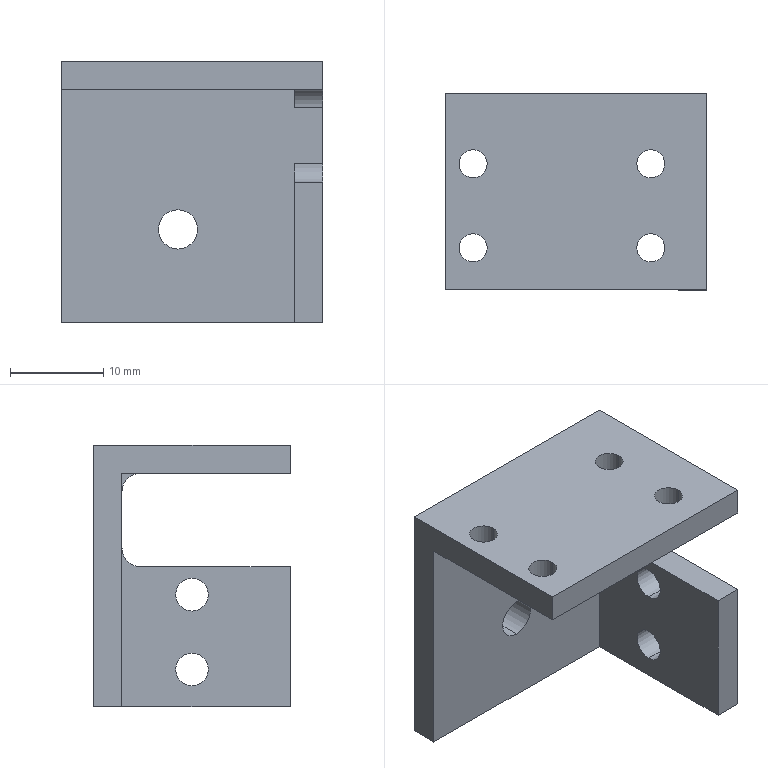Part | SolidWorks | features ICE 2, Extrusion 1 | 1 solid | 28 faces | box 28 x 21 x 28 mm | volume 4495 mm3 | cylinder 16 | plane 12 | commonest cylinder face diameters 3 x8 3.5 x4 4 x2 4.2 x2
STEP:
#1=CARTESIAN_POINT('',(15.5,1.5,-14.75));
#2=VERTEX_POINT('',#1);
#3=CARTESIAN_POINT('',(15.5,1.5,-11.25));
#4=VERTEX_POINT('',#3);
#5=CARTESIAN_POINT('',(15.5,1.5,-13.));
#6=DIRECTION('',(-1.,0.,0.));
#7=DIRECTION('',(0.,0.,1.));
#8=AXIS2_PLACEMENT_3D('',#5,#6,#7);
#9=CIRCLE('',#8,1.75);
#10=EDGE_CURVE('',#2,#4,#9,.T.);
#11=ORIENTED_EDGE('',*,*,#10,.F.);
#12=CARTESIAN_POINT('',(12.5,1.5,-14.75));
#13=VERTEX_POINT('',#12);
#14=CARTESIAN_POINT('',(15.5,1.5,-14.75));
#15=DIRECTION('',(-1.,0.,0.));
#16=VECTOR('',#15,1000.);
#17=LINE('',#14,#16);
#18=EDGE_CURVE('',#2,#13,#17,.T.);
#19=ORIENTED_EDGE('',*,*,#18,.T.);
#20=CARTESIAN_POINT('',(12.5,1.5,-11.25));
#21=VERTEX_POINT('',#20);
#22=CARTESIAN_POINT('',(12.5,1.5,-13.));
#23=DIRECTION('',(-1.,0.,0.));
#24=DIRECTION('',(0.,0.,1.));
#25=AXIS2_PLACEMENT_3D('',#22,#23,#24);
#26=CIRCLE('',#25,1.75);
#27=EDGE_CURVE('',#13,#21,#26,.T.);
#28=ORIENTED_EDGE('',*,*,#27,.T.);
#29=CARTESIAN_POINT('',(15.5,1.5,-11.25));
#30=DIRECTION('',(-1.,0.,0.));
#31=VECTOR('',#30,1000.);
#32=LINE('',#29,#31);
#33=EDGE_CURVE('',#4,#21,#32,.T.);
#34=ORIENTED_EDGE('',*,*,#33,.F.);
#35=EDGE_LOOP('',(#11,#19,#28,#34));
#36=FACE_OUTER_BOUND('',#35,.T.);
#37=CARTESIAN_POINT('',(15.5,1.5,-13.));
#38=DIRECTION('',(-1.,0.,0.));
#39=DIRECTION('',(0.,0.,1.));
#40=AXIS2_PLACEMENT_3D('',#37,#38,#39);
#41=CYLINDRICAL_SURFACE('',#40,1.75);
#42=ADVANCED_FACE('',(#36),#41,.F.);
#43=CARTESIAN_POINT('',(15.5,1.5,-22.75));
#44=VERTEX_POINT('',#43);
#45=CARTESIAN_POINT('',(15.5,1.5,-19.25));
#46=VERTEX_POINT('',#45);
#47=CARTESIAN_POINT('',(15.5,1.5,-21.));
#48=DIRECTION('',(-1.,0.,0.));
#49=DIRECTION('',(0.,0.,1.));
#50=AXIS2_PLACEMENT_3D('',#47,#48,#49);
#51=CIRCLE('',#50,1.75);
#52=EDGE_CURVE('',#44,#46,#51,.T.);
#53=ORIENTED_EDGE('',*,*,#52,.F.);
#54=CARTESIAN_POINT('',(12.5,1.5,-22.75));
#55=VERTEX_POINT('',#54);
#56=CARTESIAN_POINT('',(15.5,1.5,-22.75));
#57=DIRECTION('',(-1.,0.,0.));
#58=VECTOR('',#57,1000.);
#59=LINE('',#56,#58);
#60=EDGE_CURVE('',#44,#55,#59,.T.);
#61=ORIENTED_EDGE('',*,*,#60,.T.);
#62=CARTESIAN_POINT('',(12.5,1.5,-19.25));
#63=VERTEX_POINT('',#62);
#64=CARTESIAN_POINT('',(12.5,1.5,-21.));
#65=DIRECTION('',(-1.,0.,0.));
#66=DIRECTION('',(0.,0.,1.));
#67=AXIS2_PLACEMENT_3D('',#64,#65,#66);
#68=CIRCLE('',#67,1.75);
#69=EDGE_CURVE('',#55,#63,#68,.T.);
#70=ORIENTED_EDGE('',*,*,#69,.T.);
#71=CARTESIAN_POINT('',(15.5,1.5,-19.25));
#72=DIRECTION('',(-1.,0.,0.));
#73=VECTOR('',#72,1000.);
#74=LINE('',#71,#73);
#75=EDGE_CURVE('',#46,#63,#74,.T.);
#76=ORIENTED_EDGE('',*,*,#75,.F.);
#77=EDGE_LOOP('',(#53,#61,#70,#76));
#78=FACE_OUTER_BOUND('',#77,.T.);
#79=CARTESIAN_POINT('',(15.5,1.5,-21.));
#80=DIRECTION('',(-1.,0.,0.));
#81=DIRECTION('',(0.,0.,1.));
#82=AXIS2_PLACEMENT_3D('',#79,#80,#81);
#83=CYLINDRICAL_SURFACE('',#82,1.75);
#84=ADVANCED_FACE('',(#78),#83,.F.);
#85=CARTESIAN_POINT('',(0.,12.,-17.1));
#86=VERTEX_POINT('',#85);
#87=CARTESIAN_POINT('',(0.,12.,-12.9));
#88=VERTEX_POINT('',#87);
#89=CARTESIAN_POINT('',(0.,12.,-15.));
#90=DIRECTION('',(0.,1.,0.));
#91=DIRECTION('',(0.,0.,1.));
#92=AXIS2_PLACEMENT_3D('',#89,#90,#91);
#93=CIRCLE('',#92,2.1);
#94=EDGE_CURVE('',#86,#88,#93,.T.);
#95=ORIENTED_EDGE('',*,*,#94,.T.);
#96=CARTESIAN_POINT('',(0.,9.,-12.9));
#97=VERTEX_POINT('',#96);
#98=CARTESIAN_POINT('',(0.,12.,-12.9));
#99=DIRECTION('',(0.,-1.,0.));
#100=VECTOR('',#99,1000.);
#101=LINE('',#98,#100);
#102=EDGE_CURVE('',#88,#97,#101,.T.);
#103=ORIENTED_EDGE('',*,*,#102,.T.);
#104=CARTESIAN_POINT('',(0.,9.,-17.1));
#105=VERTEX_POINT('',#104);
#106=CARTESIAN_POINT('',(0.,9.,-15.));
#107=DIRECTION('',(0.,1.,0.));
#108=DIRECTION('',(0.,0.,1.));
#109=AXIS2_PLACEMENT_3D('',#106,#107,#108);
#110=CIRCLE('',#109,2.1);
#111=EDGE_CURVE('',#105,#97,#110,.T.);
#112=ORIENTED_EDGE('',*,*,#111,.F.);
#113=CARTESIAN_POINT('',(0.,12.,-17.1));
#114=DIRECTION('',(0.,-1.,0.));
#115=VECTOR('',#114,1000.);
#116=LINE('',#113,#115);
#117=EDGE_CURVE('',#86,#105,#116,.T.);
#118=ORIENTED_EDGE('',*,*,#117,.F.);
#119=EDGE_LOOP('',(#95,#103,#112,#118));
#120=FACE_OUTER_BOUND('',#119,.T.);
#121=CARTESIAN_POINT('',(0.,12.,-15.));
#122=DIRECTION('',(0.,-1.,0.));
#123=DIRECTION('',(0.,0.,-1.));
#124=AXIS2_PLACEMENT_3D('',#121,#122,#123);
#125=CYLINDRICAL_SURFACE('',#124,2.1);
#126=ADVANCED_FACE('',(#120),#125,.F.);
#127=CARTESIAN_POINT('',(-11.,-4.5,3.));
#128=VERTEX_POINT('',#127);
#129=CARTESIAN_POINT('',(-8.,-4.5,3.));
#130=VERTEX_POINT('',#129);
#131=CARTESIAN_POINT('',(-9.5,-4.5,3.));
#132=DIRECTION('',(0.,0.,1.));
#133=DIRECTION('',(1.,0.,0.));
#134=AXIS2_PLACEMENT_3D('',#131,#132,#133);
#135=CIRCLE('',#134,1.5);
#136=EDGE_CURVE('',#128,#130,#135,.T.);
#137=ORIENTED_EDGE('',*,*,#136,.T.);
#138=CARTESIAN_POINT('',(-8.,-4.5,0.));
#139=VERTEX_POINT('',#138);
#140=CARTESIAN_POINT('',(-8.,-4.5,3.));
#141=DIRECTION('',(0.,0.,-1.));
#142=VECTOR('',#141,1000.);
#143=LINE('',#140,#142);
#144=EDGE_CURVE('',#130,#139,#143,.T.);
#145=ORIENTED_EDGE('',*,*,#144,.T.);
#146=CARTESIAN_POINT('',(-11.,-4.5,0.));
#147=VERTEX_POINT('',#146);
#148=CARTESIAN_POINT('',(-9.5,-4.5,0.));
#149=DIRECTION('',(0.,0.,1.));
#150=DIRECTION('',(1.,0.,0.));
#151=AXIS2_PLACEMENT_3D('',#148,#149,#150);
#152=CIRCLE('',#151,1.5);
#153=EDGE_CURVE('',#147,#139,#152,.T.);
#154=ORIENTED_EDGE('',*,*,#153,.F.);
#155=CARTESIAN_POINT('',(-11.,-4.5,3.));
#156=DIRECTION('',(0.,0.,-1.));
#157=VECTOR('',#156,1000.);
#158=LINE('',#155,#157);
#159=EDGE_CURVE('',#128,#147,#158,.T.);
#160=ORIENTED_EDGE('',*,*,#159,.F.);
#161=EDGE_LOOP('',(#137,#145,#154,#160));
#162=FACE_OUTER_BOUND('',#161,.T.);
#163=CARTESIAN_POINT('',(-9.5,-4.5,3.));
#164=DIRECTION('',(0.,0.,-1.));
#165=DIRECTION('',(-1.,0.,0.));
#166=AXIS2_PLACEMENT_3D('',#163,#164,#165);
#167=CYLINDRICAL_SURFACE('',#166,1.5);
#168=ADVANCED_FACE('',(#162),#167,.F.);
#169=CARTESIAN_POINT('',(8.,-4.5,3.));
#170=VERTEX_POINT('',#169);
#171=CARTESIAN_POINT('',(11.,-4.5,3.));
#172=VERTEX_POINT('',#171);
#173=CARTESIAN_POINT('',(9.5,-4.5,3.));
#174=DIRECTION('',(0.,0.,1.));
#175=DIRECTION('',(1.,0.,0.));
#176=AXIS2_PLACEMENT_3D('',#173,#174,#175);
#177=CIRCLE('',#176,1.5);
#178=EDGE_CURVE('',#170,#172,#177,.T.);
#179=ORIENTED_EDGE('',*,*,#178,.T.);
#180=CARTESIAN_POINT('',(11.,-4.5,0.));
#181=VERTEX_POINT('',#180);
#182=CARTESIAN_POINT('',(11.,-4.5,3.));
#183=DIRECTION('',(0.,0.,-1.));
#184=VECTOR('',#183,1000.);
#185=LINE('',#182,#184);
#186=EDGE_CURVE('',#172,#181,#185,.T.);
#187=ORIENTED_EDGE('',*,*,#186,.T.);
#188=CARTESIAN_POINT('',(8.,-4.5,0.));
#189=VERTEX_POINT('',#188);
#190=CARTESIAN_POINT('',(9.5,-4.5,0.));
#191=DIRECTION('',(0.,0.,1.));
#192=DIRECTION('',(1.,0.,0.));
#193=AXIS2_PLACEMENT_3D('',#190,#191,#192);
#194=CIRCLE('',#193,1.5);
#195=EDGE_CURVE('',#189,#181,#194,.T.);
#196=ORIENTED_EDGE('',*,*,#195,.F.);
#197=CARTESIAN_POINT('',(8.,-4.5,3.));
#198=DIRECTION('',(0.,0.,-1.));
#199=VECTOR('',#198,1000.);
#200=LINE('',#197,#199);
#201=EDGE_CURVE('',#170,#189,#200,.T.);
#202=ORIENTED_EDGE('',*,*,#201,.F.);
#203=EDGE_LOOP('',(#179,#187,#196,#202));
#204=FACE_OUTER_BOUND('',#203,.T.);
#205=CARTESIAN_POINT('',(9.5,-4.5,3.));
#206=DIRECTION('',(0.,0.,-1.));
#207=DIRECTION('',(-1.,0.,0.));
#208=AXIS2_PLACEMENT_3D('',#205,#206,#207);
#209=CYLINDRICAL_SURFACE('',#208,1.5);
#210=ADVANCED_FACE('',(#204),#209,.F.);
#211=CARTESIAN_POINT('',(8.,4.5,3.));
#212=VERTEX_POINT('',#211);
#213=CARTESIAN_POINT('',(11.,4.5,3.));
#214=VERTEX_POINT('',#213);
#215=CARTESIAN_POINT('',(9.5,4.5,3.));
#216=DIRECTION('',(0.,0.,1.));
#217=DIRECTION('',(1.,0.,0.));
#218=AXIS2_PLACEMENT_3D('',#215,#216,#217);
#219=CIRCLE('',#218,1.5);
#220=EDGE_CURVE('',#212,#214,#219,.T.);
#221=ORIENTED_EDGE('',*,*,#220,.T.);
#222=CARTESIAN_POINT('',(11.,4.5,0.));
#223=VERTEX_POINT('',#222);
#224=CARTESIAN_POINT('',(11.,4.5,3.));
#225=DIRECTION('',(0.,0.,-1.));
#226=VECTOR('',#225,1000.);
#227=LINE('',#224,#226);
#228=EDGE_CURVE('',#214,#223,#227,.T.);
#229=ORIENTED_EDGE('',*,*,#228,.T.);
#230=CARTESIAN_POINT('',(8.,4.5,0.));
#231=VERTEX_POINT('',#230);
#232=CARTESIAN_POINT('',(9.5,4.5,0.));
#233=DIRECTION('',(0.,0.,1.));
#234=DIRECTION('',(1.,0.,0.));
#235=AXIS2_PLACEMENT_3D('',#232,#233,#234);
#236=CIRCLE('',#235,1.5);
#237=EDGE_CURVE('',#231,#223,#236,.T.);
#238=ORIENTED_EDGE('',*,*,#237,.F.);
#239=CARTESIAN_POINT('',(8.,4.5,3.));
#240=DIRECTION('',(0.,0.,-1.));
#241=VECTOR('',#240,1000.);
#242=LINE('',#239,#241);
#243=EDGE_CURVE('',#212,#231,#242,.T.);
#244=ORIENTED_EDGE('',*,*,#243,.F.);
#245=EDGE_LOOP('',(#221,#229,#238,#244));
#246=FACE_OUTER_BOUND('',#245,.T.);
#247=CARTESIAN_POINT('',(9.5,4.5,3.));
#248=DIRECTION('',(0.,0.,-1.));
#249=DIRECTION('',(-1.,0.,0.));
#250=AXIS2_PLACEMENT_3D('',#247,#248,#249);
#251=CYLINDRICAL_SURFACE('',#250,1.5);
#252=ADVANCED_FACE('',(#246),#251,.F.);
#253=CARTESIAN_POINT('',(-11.,4.5,3.));
#254=VERTEX_POINT('',#253);
#255=CARTESIAN_POINT('',(-8.,4.5,3.));
#256=VERTEX_POINT('',#255);
#257=CARTESIAN_POINT('',(-9.5,4.5,3.));
#258=DIRECTION('',(0.,0.,1.));
#259=DIRECTION('',(1.,0.,0.));
#260=AXIS2_PLACEMENT_3D('',#257,#258,#259);
#261=CIRCLE('',#260,1.5);
#262=EDGE_CURVE('',#254,#256,#261,.T.);
#263=ORIENTED_EDGE('',*,*,#262,.T.);
#264=CARTESIAN_POINT('',(-8.,4.5,0.));
#265=VERTEX_POINT('',#264);
#266=CARTESIAN_POINT('',(-8.,4.5,3.));
#267=DIRECTION('',(0.,0.,-1.));
#268=VECTOR('',#267,1000.);
#269=LINE('',#266,#268);
#270=EDGE_CURVE('',#256,#265,#269,.T.);
#271=ORIENTED_EDGE('',*,*,#270,.T.);
#272=CARTESIAN_POINT('',(-11.,4.5,0.));
#273=VERTEX_POINT('',#272);
#274=CARTESIAN_POINT('',(-9.5,4.5,0.));
#275=DIRECTION('',(0.,0.,1.));
#276=DIRECTION('',(1.,0.,0.));
#277=AXIS2_PLACEMENT_3D('',#274,#275,#276);
#278=CIRCLE('',#277,1.5);
#279=EDGE_CURVE('',#273,#265,#278,.T.);
#280=ORIENTED_EDGE('',*,*,#279,.F.);
#281=CARTESIAN_POINT('',(-11.,4.5,3.));
#282=DIRECTION('',(0.,0.,-1.));
#283=VECTOR('',#282,1000.);
#284=LINE('',#281,#283);
#285=EDGE_CURVE('',#254,#273,#284,.T.);
#286=ORIENTED_EDGE('',*,*,#285,.F.);
#287=EDGE_LOOP('',(#263,#271,#280,#286));
#288=FACE_OUTER_BOUND('',#287,.T.);
#289=CARTESIAN_POINT('',(-9.5,4.5,3.));
#290=DIRECTION('',(0.,0.,-1.));
#291=DIRECTION('',(-1.,0.,0.));
#292=AXIS2_PLACEMENT_3D('',#289,#290,#291);
#293=CYLINDRICAL_SURFACE('',#292,1.5);
#294=ADVANCED_FACE('',(#288),#293,.F.);
#295=CARTESIAN_POINT('',(-12.5,-9.,3.));
#296=VERTEX_POINT('',#295);
#297=CARTESIAN_POINT('',(15.5,-9.,3.));
#298=VERTEX_POINT('',#297);
#299=CARTESIAN_POINT('',(-12.5,-9.,3.));
#300=DIRECTION('',(1.,0.,0.));
#301=VECTOR('',#300,1000.);
#302=LINE('',#299,#301);
#303=EDGE_CURVE('',#296,#298,#302,.T.);
#304=ORIENTED_EDGE('',*,*,#303,.T.);
#305=CARTESIAN_POINT('',(15.5,12.,3.));
#306=VERTEX_POINT('',#305);
#307=CARTESIAN_POINT('',(15.5,12.,3.));
#308=DIRECTION('',(0.,1.,0.));
#309=VECTOR('',#308,1000.);
#310=LINE('',#307,#309);
#311=EDGE_CURVE('',#298,#306,#310,.T.);
#312=ORIENTED_EDGE('',*,*,#311,.T.);
#313=CARTESIAN_POINT('',(-12.5,12.,3.));
#314=VERTEX_POINT('',#313);
#315=CARTESIAN_POINT('',(-12.5,12.,3.));
#316=DIRECTION('',(1.,0.,0.));
#317=VECTOR('',#316,1000.);
#318=LINE('',#315,#317);
#319=EDGE_CURVE('',#314,#306,#318,.T.);
#320=ORIENTED_EDGE('',*,*,#319,.F.);
#321=CARTESIAN_POINT('',(-12.5,-9.,3.));
#322=DIRECTION('',(0.,-1.,0.));
#323=VECTOR('',#322,1000.);
#324=LINE('',#321,#323);
#325=EDGE_CURVE('',#314,#296,#324,.T.);
#326=ORIENTED_EDGE('',*,*,#325,.T.);
#327=EDGE_LOOP('',(#304,#312,#320,#326));
#328=FACE_OUTER_BOUND('',#327,.T.);
#329=ORIENTED_EDGE('',*,*,#262,.F.);
#330=CARTESIAN_POINT('',(-9.5,4.5,3.));
#331=DIRECTION('',(0.,0.,1.));
#332=DIRECTION('',(1.,0.,0.));
#333=AXIS2_PLACEMENT_3D('',#330,#331,#332);
#334=CIRCLE('',#333,1.5);
#335=EDGE_CURVE('',#256,#254,#334,.T.);
#336=ORIENTED_EDGE('',*,*,#335,.F.);
#337=EDGE_LOOP('',(#329,#336));
#338=FACE_BOUND('',#337,.T.);
#339=ORIENTED_EDGE('',*,*,#220,.F.);
#340=CARTESIAN_POINT('',(9.5,4.5,3.));
#341=DIRECTION('',(0.,0.,1.));
#342=DIRECTION('',(1.,0.,0.));
#343=AXIS2_PLACEMENT_3D('',#340,#341,#342);
#344=CIRCLE('',#343,1.5);
#345=EDGE_CURVE('',#214,#212,#344,.T.);
#346=ORIENTED_EDGE('',*,*,#345,.F.);
#347=EDGE_LOOP('',(#339,#346));
#348=FACE_BOUND('',#347,.T.);
#349=ORIENTED_EDGE('',*,*,#178,.F.);
#350=CARTESIAN_POINT('',(9.5,-4.5,3.));
#351=DIRECTION('',(0.,0.,1.));
#352=DIRECTION('',(1.,0.,0.));
#353=AXIS2_PLACEMENT_3D('',#350,#351,#352);
#354=CIRCLE('',#353,1.5);
#355=EDGE_CURVE('',#172,#170,#354,.T.);
#356=ORIENTED_EDGE('',*,*,#355,.F.);
#357=EDGE_LOOP('',(#349,#356));
#358=FACE_BOUND('',#357,.T.);
#359=ORIENTED_EDGE('',*,*,#136,.F.);
#360=CARTESIAN_POINT('',(-9.5,-4.5,3.));
#361=DIRECTION('',(0.,0.,1.));
#362=DIRECTION('',(1.,0.,0.));
#363=AXIS2_PLACEMENT_3D('',#360,#361,#362);
#364=CIRCLE('',#363,1.5);
#365=EDGE_CURVE('',#130,#128,#364,.T.);
#366=ORIENTED_EDGE('',*,*,#365,.F.);
#367=EDGE_LOOP('',(#359,#366));
#368=FACE_BOUND('',#367,.T.);
#369=CARTESIAN_POINT('',(0.,0.,3.));
#370=DIRECTION('',(0.,0.,-1.));
#371=DIRECTION('',(-1.,0.,0.));
#372=AXIS2_PLACEMENT_3D('',#369,#370,#371);
#373=PLANE('',#372);
#374=ADVANCED_FACE('',(#328,#338,#348,#358,#368),#373,.F.);
#375=ORIENTED_EDGE('',*,*,#195,.T.);
#376=CARTESIAN_POINT('',(9.5,-4.5,0.));
#377=DIRECTION('',(0.,0.,1.));
#378=DIRECTION('',(1.,0.,0.));
#379=AXIS2_PLACEMENT_3D('',#376,#377,#378);
#380=CIRCLE('',#379,1.5);
#381=EDGE_CURVE('',#181,#189,#380,.T.);
#382=ORIENTED_EDGE('',*,*,#381,.T.);
#383=EDGE_LOOP('',(#375,#382));
#384=FACE_BOUND('',#383,.T.);
#385=ORIENTED_EDGE('',*,*,#279,.T.);
#386=CARTESIAN_POINT('',(-9.5,4.5,0.));
#387=DIRECTION('',(0.,0.,1.));
#388=DIRECTION('',(1.,0.,0.));
#389=AXIS2_PLACEMENT_3D('',#386,#387,#388);
#390=CIRCLE('',#389,1.5);
#391=EDGE_CURVE('',#265,#273,#390,.T.);
#392=ORIENTED_EDGE('',*,*,#391,.T.);
#393=EDGE_LOOP('',(#385,#392));
#394=FACE_BOUND('',#393,.T.);
#395=CARTESIAN_POINT('',(12.5,7.,0.));
#396=VERTEX_POINT('',#395);
#397=CARTESIAN_POINT('',(12.5,9.,0.));
#398=VERTEX_POINT('',#397);
#399=CARTESIAN_POINT('',(12.5,-9.,0.));
#400=DIRECTION('',(0.,1.,0.));
#401=VECTOR('',#400,1000.);
#402=LINE('',#399,#401);
#403=EDGE_CURVE('',#396,#398,#402,.T.);
#404=ORIENTED_EDGE('',*,*,#403,.F.);
#405=CARTESIAN_POINT('',(15.5,7.,0.));
#406=VERTEX_POINT('',#405);
#407=CARTESIAN_POINT('',(15.5,7.,0.));
#408=DIRECTION('',(-1.,0.,0.));
#409=VECTOR('',#408,1000.);
#410=LINE('',#407,#409);
#411=EDGE_CURVE('',#406,#396,#410,.T.);
#412=ORIENTED_EDGE('',*,*,#411,.F.);
#413=CARTESIAN_POINT('',(15.5,-9.,0.));
#414=VERTEX_POINT('',#413);
#415=CARTESIAN_POINT('',(15.5,-9.,0.));
#416=DIRECTION('',(0.,-1.,0.));
#417=VECTOR('',#416,1000.);
#418=LINE('',#415,#417);
#419=EDGE_CURVE('',#406,#414,#418,.T.);
#420=ORIENTED_EDGE('',*,*,#419,.T.);
#421=CARTESIAN_POINT('',(-12.5,-9.,0.));
#422=VERTEX_POINT('',#421);
#423=CARTESIAN_POINT('',(-12.5,-9.,0.));
#424=DIRECTION('',(1.,0.,0.));
#425=VECTOR('',#424,1000.);
#426=LINE('',#423,#425);
#427=EDGE_CURVE('',#422,#414,#426,.T.);
#428=ORIENTED_EDGE('',*,*,#427,.F.);
#429=CARTESIAN_POINT('',(-12.5,9.,0.));
#430=VERTEX_POINT('',#429);
#431=CARTESIAN_POINT('',(-12.5,-9.,0.));
#432=DIRECTION('',(0.,-1.,0.));
#433=VECTOR('',#432,1000.);
#434=LINE('',#431,#433);
#435=EDGE_CURVE('',#430,#422,#434,.T.);
#436=ORIENTED_EDGE('',*,*,#435,.F.);
#437=CARTESIAN_POINT('',(-12.5,9.,0.));
#438=DIRECTION('',(-1.,0.,0.));
#439=VECTOR('',#438,1000.);
#440=LINE('',#437,#439);
#441=EDGE_CURVE('',#398,#430,#440,.T.);
#442=ORIENTED_EDGE('',*,*,#441,.F.);
#443=EDGE_LOOP('',(#404,#412,#420,#428,#436,#442));
#444=FACE_OUTER_BOUND('',#443,.T.);
#445=ORIENTED_EDGE('',*,*,#237,.T.);
#446=CARTESIAN_POINT('',(9.5,4.5,0.));
#447=DIRECTION('',(0.,0.,1.));
#448=DIRECTION('',(1.,0.,0.));
#449=AXIS2_PLACEMENT_3D('',#446,#447,#448);
#450=CIRCLE('',#449,1.5);
#451=EDGE_CURVE('',#223,#231,#450,.T.);
#452=ORIENTED_EDGE('',*,*,#451,.T.);
#453=EDGE_LOOP('',(#445,#452));
#454=FACE_BOUND('',#453,.T.);
#455=ORIENTED_EDGE('',*,*,#153,.T.);
#456=CARTESIAN_POINT('',(-9.5,-4.5,0.));
#457=DIRECTION('',(0.,0.,1.));
#458=DIRECTION('',(1.,0.,0.));
#459=AXIS2_PLACEMENT_3D('',#456,#457,#458);
#460=CIRCLE('',#459,1.5);
#461=EDGE_CURVE('',#139,#147,#460,.T.);
#462=ORIENTED_EDGE('',*,*,#461,.T.);
#463=EDGE_LOOP('',(#455,#462));
#464=FACE_BOUND('',#463,.T.);
#465=CARTESIAN_POINT('',(0.,0.,0.));
#466=DIRECTION('',(0.,0.,-1.));
#467=DIRECTION('',(-1.,0.,0.));
#468=AXIS2_PLACEMENT_3D('',#465,#466,#467);
#469=PLANE('',#468);
#470=ADVANCED_FACE('',(#384,#394,#444,#454,#464),#469,.T.);
#471=ORIENTED_EDGE('',*,*,#435,.T.);
#472=CARTESIAN_POINT('',(-12.5,-9.,3.));
#473=DIRECTION('',(0.,0.,-1.));
#474=VECTOR('',#473,1000.);
#475=LINE('',#472,#474);
#476=EDGE_CURVE('',#296,#422,#475,.T.);
#477=ORIENTED_EDGE('',*,*,#476,.F.);
#478=ORIENTED_EDGE('',*,*,#325,.F.);
#479=CARTESIAN_POINT('',(-12.5,12.,-25.));
#480=VERTEX_POINT('',#479);
#481=CARTESIAN_POINT('',(-12.5,12.,3.));
#482=DIRECTION('',(0.,0.,1.));
#483=VECTOR('',#482,1000.);
#484=LINE('',#481,#483);
#485=EDGE_CURVE('',#480,#314,#484,.T.);
#486=ORIENTED_EDGE('',*,*,#485,.F.);
#487=CARTESIAN_POINT('',(-12.5,9.,-25.));
#488=VERTEX_POINT('',#487);
#489=CARTESIAN_POINT('',(-12.5,12.,-25.));
#490=DIRECTION('',(0.,-1.,0.));
#491=VECTOR('',#490,1000.);
#492=LINE('',#489,#491);
#493=EDGE_CURVE('',#480,#488,#492,.T.);
#494=ORIENTED_EDGE('',*,*,#493,.T.);
#495=CARTESIAN_POINT('',(-12.5,9.,3.));
#496=DIRECTION('',(0.,0.,1.));
#497=VECTOR('',#496,1000.);
#498=LINE('',#495,#497);
#499=EDGE_CURVE('',#488,#430,#498,.T.);
#500=ORIENTED_EDGE('',*,*,#499,.T.);
#501=EDGE_LOOP('',(#471,#477,#478,#486,#494,#500));
#502=FACE_OUTER_BOUND('',#501,.T.);
#503=CARTESIAN_POINT('',(-12.5,-9.,3.));
#504=DIRECTION('',(1.,0.,0.));
#505=DIRECTION('',(0.,0.,-1.));
#506=AXIS2_PLACEMENT_3D('',#503,#504,#505);
#507=PLANE('',#506);
#508=ADVANCED_FACE('',(#502),#507,.F.);
#509=ORIENTED_EDGE('',*,*,#427,.T.);
#510=CARTESIAN_POINT('',(15.5,-9.,3.));
#511=DIRECTION('',(0.,0.,1.));
#512=VECTOR('',#511,1000.);
#513=LINE('',#510,#512);
#514=EDGE_CURVE('',#414,#298,#513,.T.);
#515=ORIENTED_EDGE('',*,*,#514,.T.);
#516=ORIENTED_EDGE('',*,*,#303,.F.);
#517=ORIENTED_EDGE('',*,*,#476,.T.);
#518=EDGE_LOOP('',(#509,#515,#516,#517));
#519=FACE_OUTER_BOUND('',#518,.T.);
#520=CARTESIAN_POINT('',(-12.5,-9.,3.));
#521=DIRECTION('',(0.,1.,0.));
#522=DIRECTION('',(0.,0.,1.));
#523=AXIS2_PLACEMENT_3D('',#520,#521,#522);
#524=PLANE('',#523);
#525=ADVANCED_FACE('',(#519),#524,.F.);
#526=ORIENTED_EDGE('',*,*,#270,.F.);
#527=ORIENTED_EDGE('',*,*,#335,.T.);
#528=ORIENTED_EDGE('',*,*,#285,.T.);
#529=ORIENTED_EDGE('',*,*,#391,.F.);
#530=EDGE_LOOP('',(#526,#527,#528,#529));
#531=FACE_OUTER_BOUND('',#530,.T.);
#532=CARTESIAN_POINT('',(-9.5,4.5,3.));
#533=DIRECTION('',(0.,0.,-1.));
#534=DIRECTION('',(-1.,0.,0.));
#535=AXIS2_PLACEMENT_3D('',#532,#533,#534);
#536=CYLINDRICAL_SURFACE('',#535,1.5);
#537=ADVANCED_FACE('',(#531),#536,.F.);
#538=ORIENTED_EDGE('',*,*,#228,.F.);
#539=ORIENTED_EDGE('',*,*,#345,.T.);
#540=ORIENTED_EDGE('',*,*,#243,.T.);
#541=ORIENTED_EDGE('',*,*,#451,.F.);
#542=EDGE_LOOP('',(#538,#539,#540,#541));
#543=FACE_OUTER_BOUND('',#542,.T.);
#544=CARTESIAN_POINT('',(9.5,4.5,3.));
#545=DIRECTION('',(0.,0.,-1.));
#546=DIRECTION('',(-1.,0.,0.));
#547=AXIS2_PLACEMENT_3D('',#544,#545,#546);
#548=CYLINDRICAL_SURFACE('',#547,1.5);
#549=ADVANCED_FACE('',(#543),#548,.F.);
#550=ORIENTED_EDGE('',*,*,#186,.F.);
#551=ORIENTED_EDGE('',*,*,#355,.T.);
#552=ORIENTED_EDGE('',*,*,#201,.T.);
#553=ORIENTED_EDGE('',*,*,#381,.F.);
#554=EDGE_LOOP('',(#550,#551,#552,#553));
#555=FACE_OUTER_BOUND('',#554,.T.);
#556=CARTESIAN_POINT('',(9.5,-4.5,3.));
#557=DIRECTION('',(0.,0.,-1.));
#558=DIRECTION('',(-1.,0.,0.));
#559=AXIS2_PLACEMENT_3D('',#556,#557,#558);
#560=CYLINDRICAL_SURFACE('',#559,1.5);
#561=ADVANCED_FACE('',(#555),#560,.F.);
#562=ORIENTED_EDGE('',*,*,#144,.F.);
#563=ORIENTED_EDGE('',*,*,#365,.T.);
#564=ORIENTED_EDGE('',*,*,#159,.T.);
#565=ORIENTED_EDGE('',*,*,#461,.F.);
#566=EDGE_LOOP('',(#562,#563,#564,#565));
#567=FACE_OUTER_BOUND('',#566,.T.);
#568=CARTESIAN_POINT('',(-9.5,-4.5,3.));
#569=DIRECTION('',(0.,0.,-1.));
#570=DIRECTION('',(-1.,0.,0.));
#571=AXIS2_PLACEMENT_3D('',#568,#569,#570);
#572=CYLINDRICAL_SURFACE('',#571,1.5);
#573=ADVANCED_FACE('',(#567),#572,.F.);
#574=ORIENTED_EDGE('',*,*,#485,.T.);
#575=ORIENTED_EDGE('',*,*,#319,.T.);
#576=CARTESIAN_POINT('',(15.5,12.,-25.));
#577=VERTEX_POINT('',#576);
#578=CARTESIAN_POINT('',(15.5,12.,3.));
#579=DIRECTION('',(0.,0.,-1.));
#580=VECTOR('',#579,1000.);
#581=LINE('',#578,#580);
#582=EDGE_CURVE('',#306,#577,#581,.T.);
#583=ORIENTED_EDGE('',*,*,#582,.T.);
#584=CARTESIAN_POINT('',(-12.5,12.,-25.));
#585=DIRECTION('',(-1.,0.,0.));
#586=VECTOR('',#585,1000.);
#587=LINE('',#584,#586);
#588=EDGE_CURVE('',#577,#480,#587,.T.);
#589=ORIENTED_EDGE('',*,*,#588,.T.);
#590=EDGE_LOOP('',(#574,#575,#583,#589));
#591=FACE_OUTER_BOUND('',#590,.T.);
#592=ORIENTED_EDGE('',*,*,#94,.F.);
#593=CARTESIAN_POINT('',(0.,12.,-15.));
#594=DIRECTION('',(0.,1.,0.));
#595=DIRECTION('',(0.,0.,1.));
#596=AXIS2_PLACEMENT_3D('',#593,#594,#595);
#597=CIRCLE('',#596,2.1);
#598=EDGE_CURVE('',#88,#86,#597,.T.);
#599=ORIENTED_EDGE('',*,*,#598,.F.);
#600=EDGE_LOOP('',(#592,#599));
#601=FACE_BOUND('',#600,.T.);
#602=CARTESIAN_POINT('',(0.,12.,0.));
#603=DIRECTION('',(0.,-1.,0.));
#604=DIRECTION('',(0.,0.,-1.));
#605=AXIS2_PLACEMENT_3D('',#602,#603,#604);
#606=PLANE('',#605);
#607=ADVANCED_FACE('',(#591,#601),#606,.F.);
#608=CARTESIAN_POINT('',(12.5,9.,-2.));
#609=VERTEX_POINT('',#608);
#610=CARTESIAN_POINT('',(12.5,9.,3.));
#611=DIRECTION('',(0.,0.,-1.));
#612=VECTOR('',#611,1000.);
#613=LINE('',#610,#612);
#614=EDGE_CURVE('',#398,#609,#613,.T.);
#615=ORIENTED_EDGE('',*,*,#614,.F.);
#616=ORIENTED_EDGE('',*,*,#441,.T.);
#617=ORIENTED_EDGE('',*,*,#499,.F.);
#618=CARTESIAN_POINT('',(12.5,9.,-25.));
#619=VERTEX_POINT('',#618);
#620=CARTESIAN_POINT('',(-12.5,9.,-25.));
#621=DIRECTION('',(-1.,0.,0.));
#622=VECTOR('',#621,1000.);
#623=LINE('',#620,#622);
#624=EDGE_CURVE('',#619,#488,#623,.T.);
#625=ORIENTED_EDGE('',*,*,#624,.F.);
#626=CARTESIAN_POINT('',(12.5,9.,-8.));
#627=VERTEX_POINT('',#626);
#628=CARTESIAN_POINT('',(12.5,9.,3.));
#629=DIRECTION('',(0.,0.,-1.));
#630=VECTOR('',#629,1000.);
#631=LINE('',#628,#630);
#632=EDGE_CURVE('',#627,#619,#631,.T.);
#633=ORIENTED_EDGE('',*,*,#632,.F.);
#634=CARTESIAN_POINT('',(15.5,9.,-8.));
#635=VERTEX_POINT('',#634);
#636=CARTESIAN_POINT('',(15.5,9.,-8.));
#637=DIRECTION('',(-1.,0.,0.));
#638=VECTOR('',#637,1000.);
#639=LINE('',#636,#638);
#640=EDGE_CURVE('',#635,#627,#639,.T.);
#641=ORIENTED_EDGE('',*,*,#640,.F.);
#642=CARTESIAN_POINT('',(15.5,9.,-2.));
#643=VERTEX_POINT('',#642);
#644=CARTESIAN_POINT('',(15.5,9.,-8.));
#645=DIRECTION('',(0.,0.,1.));
#646=VECTOR('',#645,1000.);
#647=LINE('',#644,#646);
#648=EDGE_CURVE('',#635,#643,#647,.T.);
#649=ORIENTED_EDGE('',*,*,#648,.T.);
#650=CARTESIAN_POINT('',(15.5,9.,-2.));
#651=DIRECTION('',(-1.,0.,0.));
#652=VECTOR('',#651,1000.);
#653=LINE('',#650,#652);
#654=EDGE_CURVE('',#643,#609,#653,.T.);
#655=ORIENTED_EDGE('',*,*,#654,.T.);
#656=EDGE_LOOP('',(#615,#616,#617,#625,#633,#641,#649,#655));
#657=FACE_OUTER_BOUND('',#656,.T.);
#658=ORIENTED_EDGE('',*,*,#111,.T.);
#659=CARTESIAN_POINT('',(0.,9.,-15.));
#660=DIRECTION('',(0.,1.,0.));
#661=DIRECTION('',(0.,0.,1.));
#662=AXIS2_PLACEMENT_3D('',#659,#660,#661);
#663=CIRCLE('',#662,2.1);
#664=EDGE_CURVE('',#97,#105,#663,.T.);
#665=ORIENTED_EDGE('',*,*,#664,.T.);
#666=EDGE_LOOP('',(#658,#665));
#667=FACE_BOUND('',#666,.T.);
#668=CARTESIAN_POINT('',(0.,9.,0.));
#669=DIRECTION('',(0.,-1.,0.));
#670=DIRECTION('',(0.,0.,-1.));
#671=AXIS2_PLACEMENT_3D('',#668,#669,#670);
#672=PLANE('',#671);
#673=ADVANCED_FACE('',(#657,#667),#672,.T.);
#674=ORIENTED_EDGE('',*,*,#624,.T.);
#675=ORIENTED_EDGE('',*,*,#493,.F.);
#676=ORIENTED_EDGE('',*,*,#588,.F.);
#677=CARTESIAN_POINT('',(15.5,-9.,-25.));
#678=VERTEX_POINT('',#677);
#679=CARTESIAN_POINT('',(15.5,12.,-25.));
#680=DIRECTION('',(0.,-1.,0.));
#681=VECTOR('',#680,1000.);
#682=LINE('',#679,#681);
#683=EDGE_CURVE('',#577,#678,#682,.T.);
#684=ORIENTED_EDGE('',*,*,#683,.T.);
#685=CARTESIAN_POINT('',(12.5,-9.,-25.));
#686=VERTEX_POINT('',#685);
#687=CARTESIAN_POINT('',(15.5,-9.,-25.));
#688=DIRECTION('',(-1.,0.,0.));
#689=VECTOR('',#688,1000.);
#690=LINE('',#687,#689);
#691=EDGE_CURVE('',#678,#686,#690,.T.);
#692=ORIENTED_EDGE('',*,*,#691,.T.);
#693=CARTESIAN_POINT('',(12.5,12.,-25.));
#694=DIRECTION('',(0.,-1.,0.));
#695=VECTOR('',#694,1000.);
#696=LINE('',#693,#695);
#697=EDGE_CURVE('',#619,#686,#696,.T.);
#698=ORIENTED_EDGE('',*,*,#697,.F.);
#699=EDGE_LOOP('',(#674,#675,#676,#684,#692,#698));
#700=FACE_OUTER_BOUND('',#699,.T.);
#701=CARTESIAN_POINT('',(-12.5,12.,-25.));
#702=DIRECTION('',(0.,0.,1.));
#703=DIRECTION('',(1.,0.,0.));
#704=AXIS2_PLACEMENT_3D('',#701,#702,#703);
#705=PLANE('',#704);
#706=ADVANCED_FACE('',(#700),#705,.F.);
#707=ORIENTED_EDGE('',*,*,#102,.F.);
#708=ORIENTED_EDGE('',*,*,#598,.T.);
#709=ORIENTED_EDGE('',*,*,#117,.T.);
#710=ORIENTED_EDGE('',*,*,#664,.F.);
#711=EDGE_LOOP('',(#707,#708,#709,#710));
#712=FACE_OUTER_BOUND('',#711,.T.);
#713=CARTESIAN_POINT('',(0.,12.,-15.));
#714=DIRECTION('',(0.,-1.,0.));
#715=DIRECTION('',(0.,0.,-1.));
#716=AXIS2_PLACEMENT_3D('',#713,#714,#715);
#717=CYLINDRICAL_SURFACE('',#716,2.1);
#718=ADVANCED_FACE('',(#712),#717,.F.);
#719=CARTESIAN_POINT('',(12.5,7.,-2.));
#720=DIRECTION('',(1.,0.,0.));
#721=DIRECTION('',(0.,0.,-1.));
#722=AXIS2_PLACEMENT_3D('',#719,#720,#721);
#723=CIRCLE('',#722,2.);
#724=EDGE_CURVE('',#609,#396,#723,.T.);
#725=ORIENTED_EDGE('',*,*,#724,.T.);
#726=ORIENTED_EDGE('',*,*,#403,.T.);
#727=ORIENTED_EDGE('',*,*,#614,.T.);
#728=EDGE_LOOP('',(#725,#726,#727));
#729=FACE_OUTER_BOUND('',#728,.T.);
#730=CARTESIAN_POINT('',(12.5,7.,-2.));
#731=DIRECTION('',(1.,0.,0.));
#732=DIRECTION('',(0.,0.,-1.));
#733=AXIS2_PLACEMENT_3D('',#730,#731,#732);
#734=PLANE('',#733);
#735=ADVANCED_FACE('',(#729),#734,.F.);
#736=ORIENTED_EDGE('',*,*,#724,.F.);
#737=ORIENTED_EDGE('',*,*,#654,.F.);
#738=CARTESIAN_POINT('',(15.5,7.,-2.));
#739=DIRECTION('',(1.,0.,0.));
#740=DIRECTION('',(0.,0.,-1.));
#741=AXIS2_PLACEMENT_3D('',#738,#739,#740);
#742=CIRCLE('',#741,2.);
#743=EDGE_CURVE('',#643,#406,#742,.T.);
#744=ORIENTED_EDGE('',*,*,#743,.T.);
#745=ORIENTED_EDGE('',*,*,#411,.T.);
#746=EDGE_LOOP('',(#736,#737,#744,#745));
#747=FACE_OUTER_BOUND('',#746,.T.);
#748=CARTESIAN_POINT('',(15.5,7.,-2.));
#749=DIRECTION('',(-1.,0.,0.));
#750=DIRECTION('',(0.,0.,1.));
#751=AXIS2_PLACEMENT_3D('',#748,#749,#750);
#752=CYLINDRICAL_SURFACE('',#751,2.);
#753=ADVANCED_FACE('',(#747),#752,.F.);
#754=CARTESIAN_POINT('',(12.5,7.,-10.));
#755=VERTEX_POINT('',#754);
#756=CARTESIAN_POINT('',(12.5,7.,-8.));
#757=DIRECTION('',(1.,0.,0.));
#758=DIRECTION('',(0.,0.,1.));
#759=AXIS2_PLACEMENT_3D('',#756,#757,#758);
#760=CIRCLE('',#759,2.);
#761=EDGE_CURVE('',#755,#627,#760,.T.);
#762=ORIENTED_EDGE('',*,*,#761,.F.);
#763=CARTESIAN_POINT('',(15.5,7.,-10.));
#764=VERTEX_POINT('',#763);
#765=CARTESIAN_POINT('',(15.5,7.,-10.));
#766=DIRECTION('',(-1.,0.,0.));
#767=VECTOR('',#766,1000.);
#768=LINE('',#765,#767);
#769=EDGE_CURVE('',#764,#755,#768,.T.);
#770=ORIENTED_EDGE('',*,*,#769,.F.);
#771=CARTESIAN_POINT('',(15.5,7.,-8.));
#772=DIRECTION('',(1.,0.,0.));
#773=DIRECTION('',(0.,0.,1.));
#774=AXIS2_PLACEMENT_3D('',#771,#772,#773);
#775=CIRCLE('',#774,2.);
#776=EDGE_CURVE('',#764,#635,#775,.T.);
#777=ORIENTED_EDGE('',*,*,#776,.T.);
#778=ORIENTED_EDGE('',*,*,#640,.T.);
#779=EDGE_LOOP('',(#762,#770,#777,#778));
#780=FACE_OUTER_BOUND('',#779,.T.);
#781=CARTESIAN_POINT('',(15.5,7.,-8.));
#782=DIRECTION('',(-1.,0.,0.));
#783=DIRECTION('',(0.,0.,1.));
#784=AXIS2_PLACEMENT_3D('',#781,#782,#783);
#785=CYLINDRICAL_SURFACE('',#784,2.);
#786=ADVANCED_FACE('',(#780),#785,.F.);
#787=CARTESIAN_POINT('',(12.5,-9.,-10.));
#788=VERTEX_POINT('',#787);
#789=CARTESIAN_POINT('',(12.5,7.,-10.));
#790=DIRECTION('',(0.,1.,0.));
#791=VECTOR('',#790,1000.);
#792=LINE('',#789,#791);
#793=EDGE_CURVE('',#788,#755,#792,.T.);
#794=ORIENTED_EDGE('',*,*,#793,.F.);
#795=CARTESIAN_POINT('',(15.5,-9.,-10.));
#796=VERTEX_POINT('',#795);
#797=CARTESIAN_POINT('',(15.5,-9.,-10.));
#798=DIRECTION('',(-1.,0.,0.));
#799=VECTOR('',#798,1000.);
#800=LINE('',#797,#799);
#801=EDGE_CURVE('',#796,#788,#800,.T.);
#802=ORIENTED_EDGE('',*,*,#801,.F.);
#803=CARTESIAN_POINT('',(15.5,7.,-10.));
#804=DIRECTION('',(0.,1.,0.));
#805=VECTOR('',#804,1000.);
#806=LINE('',#803,#805);
#807=EDGE_CURVE('',#796,#764,#806,.T.);
#808=ORIENTED_EDGE('',*,*,#807,.T.);
#809=ORIENTED_EDGE('',*,*,#769,.T.);
#810=EDGE_LOOP('',(#794,#802,#808,#809));
#811=FACE_OUTER_BOUND('',#810,.T.);
#812=CARTESIAN_POINT('',(15.5,7.,-10.));
#813=DIRECTION('',(0.,0.,1.));
#814=DIRECTION('',(0.,-1.,0.));
#815=AXIS2_PLACEMENT_3D('',#812,#813,#814);
#816=PLANE('',#815);
#817=ADVANCED_FACE('',(#811),#816,.T.);
#818=CARTESIAN_POINT('',(12.5,-9.,-10.));
#819=DIRECTION('',(0.,0.,1.));
#820=VECTOR('',#819,1000.);
#821=LINE('',#818,#820);
#822=EDGE_CURVE('',#686,#788,#821,.T.);
#823=ORIENTED_EDGE('',*,*,#822,.F.);
#824=ORIENTED_EDGE('',*,*,#691,.F.);
#825=CARTESIAN_POINT('',(15.5,-9.,-10.));
#826=DIRECTION('',(0.,0.,1.));
#827=VECTOR('',#826,1000.);
#828=LINE('',#825,#827);
#829=EDGE_CURVE('',#678,#796,#828,.T.);
#830=ORIENTED_EDGE('',*,*,#829,.T.);
#831=ORIENTED_EDGE('',*,*,#801,.T.);
#832=EDGE_LOOP('',(#823,#824,#830,#831));
#833=FACE_OUTER_BOUND('',#832,.T.);
#834=CARTESIAN_POINT('',(15.5,-9.,-10.));
#835=DIRECTION('',(0.,-1.,0.));
#836=DIRECTION('',(0.,0.,-1.));
#837=AXIS2_PLACEMENT_3D('',#834,#835,#836);
#838=PLANE('',#837);
#839=ADVANCED_FACE('',(#833),#838,.T.);
#840=CARTESIAN_POINT('',(15.5,1.5,-13.));
#841=DIRECTION('',(-1.,0.,0.));
#842=DIRECTION('',(0.,0.,1.));
#843=AXIS2_PLACEMENT_3D('',#840,#841,#842);
#844=CIRCLE('',#843,1.75);
#845=EDGE_CURVE('',#4,#2,#844,.T.);
#846=ORIENTED_EDGE('',*,*,#845,.T.);
#847=ORIENTED_EDGE('',*,*,#10,.T.);
#848=EDGE_LOOP('',(#846,#847));
#849=FACE_BOUND('',#848,.T.);
#850=CARTESIAN_POINT('',(15.5,1.5,-21.));
#851=DIRECTION('',(-1.,0.,0.));
#852=DIRECTION('',(0.,0.,1.));
#853=AXIS2_PLACEMENT_3D('',#850,#851,#852);
#854=CIRCLE('',#853,1.75);
#855=EDGE_CURVE('',#46,#44,#854,.T.);
#856=ORIENTED_EDGE('',*,*,#855,.T.);
#857=ORIENTED_EDGE('',*,*,#52,.T.);
#858=EDGE_LOOP('',(#856,#857));
#859=FACE_BOUND('',#858,.T.);
#860=ORIENTED_EDGE('',*,*,#311,.F.);
#861=ORIENTED_EDGE('',*,*,#514,.F.);
#862=ORIENTED_EDGE('',*,*,#419,.F.);
#863=ORIENTED_EDGE('',*,*,#743,.F.);
#864=ORIENTED_EDGE('',*,*,#648,.F.);
#865=ORIENTED_EDGE('',*,*,#776,.F.);
#866=ORIENTED_EDGE('',*,*,#807,.F.);
#867=ORIENTED_EDGE('',*,*,#829,.F.);
#868=ORIENTED_EDGE('',*,*,#683,.F.);
#869=ORIENTED_EDGE('',*,*,#582,.F.);
#870=EDGE_LOOP('',(#860,#861,#862,#863,#864,#865,#866,#867,#868,#869));
#871=FACE_OUTER_BOUND('',#870,.T.);
#872=CARTESIAN_POINT('',(15.5,7.,-2.));
#873=DIRECTION('',(1.,0.,0.));
#874=DIRECTION('',(0.,0.,-1.));
#875=AXIS2_PLACEMENT_3D('',#872,#873,#874);
#876=PLANE('',#875);
#877=ADVANCED_FACE('',(#849,#859,#871),#876,.T.);
#878=CARTESIAN_POINT('',(12.5,1.5,-13.));
#879=DIRECTION('',(-1.,0.,0.));
#880=DIRECTION('',(0.,0.,1.));
#881=AXIS2_PLACEMENT_3D('',#878,#879,#880);
#882=CIRCLE('',#881,1.75);
#883=EDGE_CURVE('',#21,#13,#882,.T.);
#884=ORIENTED_EDGE('',*,*,#883,.F.);
#885=ORIENTED_EDGE('',*,*,#27,.F.);
#886=EDGE_LOOP('',(#884,#885));
#887=FACE_BOUND('',#886,.T.);
#888=CARTESIAN_POINT('',(12.5,1.5,-21.));
#889=DIRECTION('',(-1.,0.,0.));
#890=DIRECTION('',(0.,0.,1.));
#891=AXIS2_PLACEMENT_3D('',#888,#889,#890);
#892=CIRCLE('',#891,1.75);
#893=EDGE_CURVE('',#63,#55,#892,.T.);
#894=ORIENTED_EDGE('',*,*,#893,.F.);
#895=ORIENTED_EDGE('',*,*,#69,.F.);
#896=EDGE_LOOP('',(#894,#895));
#897=FACE_BOUND('',#896,.T.);
#898=ORIENTED_EDGE('',*,*,#761,.T.);
#899=ORIENTED_EDGE('',*,*,#632,.T.);
#900=ORIENTED_EDGE('',*,*,#697,.T.);
#901=ORIENTED_EDGE('',*,*,#822,.T.);
#902=ORIENTED_EDGE('',*,*,#793,.T.);
#903=EDGE_LOOP('',(#898,#899,#900,#901,#902));
#904=FACE_OUTER_BOUND('',#903,.T.);
#905=CARTESIAN_POINT('',(12.5,7.,-2.));
#906=DIRECTION('',(1.,0.,0.));
#907=DIRECTION('',(0.,0.,-1.));
#908=AXIS2_PLACEMENT_3D('',#905,#906,#907);
#909=PLANE('',#908);
#910=ADVANCED_FACE('',(#887,#897,#904),#909,.F.);
#911=ORIENTED_EDGE('',*,*,#60,.F.);
#912=ORIENTED_EDGE('',*,*,#855,.F.);
#913=ORIENTED_EDGE('',*,*,#75,.T.);
#914=ORIENTED_EDGE('',*,*,#893,.T.);
#915=EDGE_LOOP('',(#911,#912,#913,#914));
#916=FACE_OUTER_BOUND('',#915,.T.);
#917=CARTESIAN_POINT('',(15.5,1.5,-21.));
#918=DIRECTION('',(-1.,0.,0.));
#919=DIRECTION('',(0.,0.,1.));
#920=AXIS2_PLACEMENT_3D('',#917,#918,#919);
#921=CYLINDRICAL_SURFACE('',#920,1.75);
#922=ADVANCED_FACE('',(#916),#921,.F.);
#923=ORIENTED_EDGE('',*,*,#18,.F.);
#924=ORIENTED_EDGE('',*,*,#845,.F.);
#925=ORIENTED_EDGE('',*,*,#33,.T.);
#926=ORIENTED_EDGE('',*,*,#883,.T.);
#927=EDGE_LOOP('',(#923,#924,#925,#926));
#928=FACE_OUTER_BOUND('',#927,.T.);
#929=CARTESIAN_POINT('',(15.5,1.5,-13.));
#930=DIRECTION('',(-1.,0.,0.));
#931=DIRECTION('',(0.,0.,1.));
#932=AXIS2_PLACEMENT_3D('',#929,#930,#931);
#933=CYLINDRICAL_SURFACE('',#932,1.75);
#934=ADVANCED_FACE('',(#928),#933,.F.);
#935=CLOSED_SHELL('',(#42,#84,#126,#168,#210,#252,#294,#374,#470,#508,#525,#537,#549,#561,#573,#607,#673,#706,#718,#735,#753,#786,#817,#839,#877,#910,#922,#934));
#936=MANIFOLD_SOLID_BREP('',#935);
#937=CARTESIAN_POINT('',(0.,0.,0.));
#938=DIRECTION('',(0.,0.,1.));
#939=DIRECTION('',(1.,0.,0.));
#940=AXIS2_PLACEMENT_3D('',#937,#938,#939);
#941=(LENGTH_UNIT()NAMED_UNIT(*)SI_UNIT(.MILLI.,.METRE.));
#942=UNCERTAINTY_MEASURE_WITH_UNIT(LENGTH_MEASURE(0.00001),#941,'','');
#943=(NAMED_UNIT(*)PLANE_ANGLE_UNIT()SI_UNIT($,.RADIAN.));
#944=(NAMED_UNIT(*)SI_UNIT($,.STERADIAN.)SOLID_ANGLE_UNIT());
#945=(GEOMETRIC_REPRESENTATION_CONTEXT(3)GLOBAL_UNCERTAINTY_ASSIGNED_CONTEXT((#942))GLOBAL_UNIT_ASSIGNED_CONTEXT((#941,#943,#944))REPRESENTATION_CONTEXT('',''));
#946=ADVANCED_BREP_SHAPE_REPRESENTATION('',(#936,#940),#945);